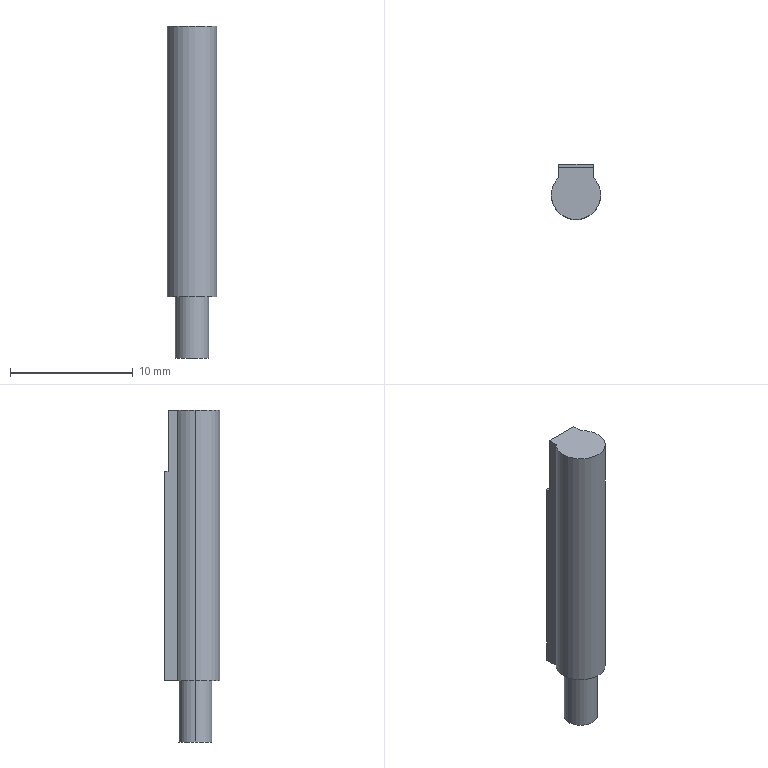Part | SolidWorks | features ICE 3, RefAxis 3, 3DProfileFeature 1, Extrusion 1, Revolution 1 | 1 solid | 23 faces | box 4 x 4.5 x 27 mm | volume 342.413 mm3 | plane 13 | cylinder 10 | commonest cylinder face diameters 2.1 x3 4 x3 2.5 x2 2.7 x2
STEP:
#1=CARTESIAN_POINT('',(1.35,0.,-27.));
#2=VERTEX_POINT('',#1);
#3=CARTESIAN_POINT('',(-1.35,0.,-27.));
#4=VERTEX_POINT('',#3);
#5=CARTESIAN_POINT('',(0.,0.,-27.));
#6=DIRECTION('',(0.,0.,1.));
#7=DIRECTION('',(1.,0.,0.));
#8=AXIS2_PLACEMENT_3D('',#5,#6,#7);
#9=CIRCLE('',#8,1.35);
#10=EDGE_CURVE('',#2,#4,#9,.T.);
#11=ORIENTED_EDGE('',*,*,#10,.T.);
#12=CARTESIAN_POINT('',(-1.35,0.,-22.));
#13=VERTEX_POINT('',#12);
#14=CARTESIAN_POINT('',(-1.35,0.,-27.));
#15=DIRECTION('',(0.,0.,1.));
#16=VECTOR('',#15,1000.);
#17=LINE('',#14,#16);
#18=EDGE_CURVE('',#4,#13,#17,.T.);
#19=ORIENTED_EDGE('',*,*,#18,.T.);
#20=CARTESIAN_POINT('',(1.35,0.,-22.));
#21=VERTEX_POINT('',#20);
#22=CARTESIAN_POINT('',(0.,0.,-22.));
#23=DIRECTION('',(0.,0.,-1.));
#24=DIRECTION('',(1.,0.,0.));
#25=AXIS2_PLACEMENT_3D('',#22,#23,#24);
#26=CIRCLE('',#25,1.35);
#27=EDGE_CURVE('',#13,#21,#26,.T.);
#28=ORIENTED_EDGE('',*,*,#27,.T.);
#29=CARTESIAN_POINT('',(1.35,0.,-27.));
#30=DIRECTION('',(0.,0.,1.));
#31=VECTOR('',#30,1000.);
#32=LINE('',#29,#31);
#33=EDGE_CURVE('',#2,#21,#32,.T.);
#34=ORIENTED_EDGE('',*,*,#33,.F.);
#35=EDGE_LOOP('',(#11,#19,#28,#34));
#36=FACE_OUTER_BOUND('',#35,.T.);
#37=CARTESIAN_POINT('',(0.,0.,-27.));
#38=DIRECTION('',(0.,0.,1.));
#39=DIRECTION('',(1.,0.,0.));
#40=AXIS2_PLACEMENT_3D('',#37,#38,#39);
#41=CYLINDRICAL_SURFACE('',#40,1.35);
#42=ADVANCED_FACE('',(#36),#41,.T.);
#43=CARTESIAN_POINT('',(-0.5443,2.1,-1.102));
#44=VERTEX_POINT('',#43);
#45=CARTESIAN_POINT('',(0.,2.1,-0.95));
#46=VERTEX_POINT('',#45);
#47=CARTESIAN_POINT('',(0.,2.1,-2.));
#48=DIRECTION('',(0.,1.,0.));
#49=DIRECTION('',(0.,0.,1.));
#50=AXIS2_PLACEMENT_3D('',#47,#48,#49);
#51=CIRCLE('',#50,1.05);
#52=EDGE_CURVE('',#44,#46,#51,.T.);
#53=ORIENTED_EDGE('',*,*,#52,.T.);
#54=CARTESIAN_POINT('',(0.,2.2,-0.95));
#55=VERTEX_POINT('',#54);
#56=CARTESIAN_POINT('',(0.,2.1,-0.95));
#57=DIRECTION('',(0.,1.,0.));
#58=VECTOR('',#57,1000.);
#59=LINE('',#56,#58);
#60=EDGE_CURVE('',#46,#55,#59,.T.);
#61=ORIENTED_EDGE('',*,*,#60,.T.);
#62=CARTESIAN_POINT('',(-0.5443,2.2,-1.102));
#63=VERTEX_POINT('',#62);
#64=CARTESIAN_POINT('',(0.,2.2,-2.));
#65=DIRECTION('',(0.,1.,0.));
#66=DIRECTION('',(0.,0.,1.));
#67=AXIS2_PLACEMENT_3D('',#64,#65,#66);
#68=CIRCLE('',#67,1.05);
#69=EDGE_CURVE('',#63,#55,#68,.T.);
#70=ORIENTED_EDGE('',*,*,#69,.F.);
#71=CARTESIAN_POINT('',(-0.5443,2.1,-1.102));
#72=DIRECTION('',(0.,1.,0.));
#73=VECTOR('',#72,1000.);
#74=LINE('',#71,#73);
#75=EDGE_CURVE('',#44,#63,#74,.T.);
#76=ORIENTED_EDGE('',*,*,#75,.F.);
#77=EDGE_LOOP('',(#53,#61,#70,#76));
#78=FACE_OUTER_BOUND('',#77,.T.);
#79=CARTESIAN_POINT('',(0.,2.1,-2.));
#80=DIRECTION('',(0.,1.,0.));
#81=DIRECTION('',(0.,0.,1.));
#82=AXIS2_PLACEMENT_3D('',#79,#80,#81);
#83=CYLINDRICAL_SURFACE('',#82,1.05);
#84=ADVANCED_FACE('',(#78),#83,.T.);
#85=CARTESIAN_POINT('',(0.,2.1,-3.25));
#86=VERTEX_POINT('',#85);
#87=CARTESIAN_POINT('',(0.,2.1,-0.75));
#88=VERTEX_POINT('',#87);
#89=CARTESIAN_POINT('',(0.,2.1,-2.));
#90=DIRECTION('',(0.,1.,0.));
#91=DIRECTION('',(0.,0.,1.));
#92=AXIS2_PLACEMENT_3D('',#89,#90,#91);
#93=CIRCLE('',#92,1.25);
#94=EDGE_CURVE('',#86,#88,#93,.T.);
#95=ORIENTED_EDGE('',*,*,#94,.F.);
#96=CARTESIAN_POINT('',(0.,2.2,-3.25));
#97=VERTEX_POINT('',#96);
#98=CARTESIAN_POINT('',(0.,2.1,-3.25));
#99=DIRECTION('',(0.,1.,0.));
#100=VECTOR('',#99,1000.);
#101=LINE('',#98,#100);
#102=EDGE_CURVE('',#86,#97,#101,.T.);
#103=ORIENTED_EDGE('',*,*,#102,.T.);
#104=CARTESIAN_POINT('',(0.,2.2,-0.75));
#105=VERTEX_POINT('',#104);
#106=CARTESIAN_POINT('',(0.,2.2,-2.));
#107=DIRECTION('',(0.,1.,0.));
#108=DIRECTION('',(0.,0.,1.));
#109=AXIS2_PLACEMENT_3D('',#106,#107,#108);
#110=CIRCLE('',#109,1.25);
#111=EDGE_CURVE('',#97,#105,#110,.T.);
#112=ORIENTED_EDGE('',*,*,#111,.T.);
#113=CARTESIAN_POINT('',(0.,2.1,-0.75));
#114=DIRECTION('',(0.,1.,0.));
#115=VECTOR('',#114,1000.);
#116=LINE('',#113,#115);
#117=EDGE_CURVE('',#88,#105,#116,.T.);
#118=ORIENTED_EDGE('',*,*,#117,.F.);
#119=EDGE_LOOP('',(#95,#103,#112,#118));
#120=FACE_OUTER_BOUND('',#119,.T.);
#121=CARTESIAN_POINT('',(0.,2.1,-2.));
#122=DIRECTION('',(0.,1.,0.));
#123=DIRECTION('',(0.,0.,1.));
#124=AXIS2_PLACEMENT_3D('',#121,#122,#123);
#125=CYLINDRICAL_SURFACE('',#124,1.25);
#126=ADVANCED_FACE('',(#120),#125,.F.);
#127=CARTESIAN_POINT('',(-1.4,1.428,-22.));
#128=VERTEX_POINT('',#127);
#129=CARTESIAN_POINT('',(-2.,0.,-22.));
#130=VERTEX_POINT('',#129);
#131=CARTESIAN_POINT('',(0.,0.,-22.));
#132=DIRECTION('',(0.,0.,1.));
#133=DIRECTION('',(1.,0.,0.));
#134=AXIS2_PLACEMENT_3D('',#131,#132,#133);
#135=CIRCLE('',#134,2.);
#136=EDGE_CURVE('',#128,#130,#135,.T.);
#137=ORIENTED_EDGE('',*,*,#136,.T.);
#138=CARTESIAN_POINT('',(-2.,0.,0.));
#139=VERTEX_POINT('',#138);
#140=CARTESIAN_POINT('',(-2.,0.,-22.));
#141=DIRECTION('',(0.,0.,1.));
#142=VECTOR('',#141,1000.);
#143=LINE('',#140,#142);
#144=EDGE_CURVE('',#130,#139,#143,.T.);
#145=ORIENTED_EDGE('',*,*,#144,.T.);
#146=CARTESIAN_POINT('',(-1.4,1.428,0.));
#147=VERTEX_POINT('',#146);
#148=CARTESIAN_POINT('',(0.,0.,0.));
#149=DIRECTION('',(0.,0.,1.));
#150=DIRECTION('',(1.,0.,0.));
#151=AXIS2_PLACEMENT_3D('',#148,#149,#150);
#152=CIRCLE('',#151,2.);
#153=EDGE_CURVE('',#147,#139,#152,.T.);
#154=ORIENTED_EDGE('',*,*,#153,.F.);
#155=CARTESIAN_POINT('',(-1.4,1.428,-22.));
#156=DIRECTION('',(0.,0.,1.));
#157=VECTOR('',#156,1000.);
#158=LINE('',#155,#157);
#159=EDGE_CURVE('',#128,#147,#158,.T.);
#160=ORIENTED_EDGE('',*,*,#159,.F.);
#161=EDGE_LOOP('',(#137,#145,#154,#160));
#162=FACE_OUTER_BOUND('',#161,.T.);
#163=CARTESIAN_POINT('',(0.,0.,-22.));
#164=DIRECTION('',(0.,0.,1.));
#165=DIRECTION('',(1.,0.,0.));
#166=AXIS2_PLACEMENT_3D('',#163,#164,#165);
#167=CYLINDRICAL_SURFACE('',#166,2.);
#168=ADVANCED_FACE('',(#162),#167,.T.);
#169=ORIENTED_EDGE('',*,*,#144,.F.);
#170=CARTESIAN_POINT('',(2.,0.,-22.));
#171=VERTEX_POINT('',#170);
#172=CARTESIAN_POINT('',(0.,0.,-22.));
#173=DIRECTION('',(0.,0.,1.));
#174=DIRECTION('',(1.,0.,0.));
#175=AXIS2_PLACEMENT_3D('',#172,#173,#174);
#176=CIRCLE('',#175,2.);
#177=EDGE_CURVE('',#130,#171,#176,.T.);
#178=ORIENTED_EDGE('',*,*,#177,.T.);
#179=CARTESIAN_POINT('',(2.,0.,0.));
#180=VERTEX_POINT('',#179);
#181=CARTESIAN_POINT('',(2.,0.,-22.));
#182=DIRECTION('',(0.,0.,1.));
#183=VECTOR('',#182,1000.);
#184=LINE('',#181,#183);
#185=EDGE_CURVE('',#171,#180,#184,.T.);
#186=ORIENTED_EDGE('',*,*,#185,.T.);
#187=CARTESIAN_POINT('',(0.,0.,0.));
#188=DIRECTION('',(0.,0.,1.));
#189=DIRECTION('',(1.,0.,0.));
#190=AXIS2_PLACEMENT_3D('',#187,#188,#189);
#191=CIRCLE('',#190,2.);
#192=EDGE_CURVE('',#139,#180,#191,.T.);
#193=ORIENTED_EDGE('',*,*,#192,.F.);
#194=EDGE_LOOP('',(#169,#178,#186,#193));
#195=FACE_OUTER_BOUND('',#194,.T.);
#196=CARTESIAN_POINT('',(0.,0.,-22.));
#197=DIRECTION('',(0.,0.,1.));
#198=DIRECTION('',(1.,0.,0.));
#199=AXIS2_PLACEMENT_3D('',#196,#197,#198);
#200=CYLINDRICAL_SURFACE('',#199,2.);
#201=ADVANCED_FACE('',(#195),#200,.T.);
#202=ORIENTED_EDGE('',*,*,#136,.F.);
#203=CARTESIAN_POINT('',(-1.4,2.5,-22.));
#204=VERTEX_POINT('',#203);
#205=CARTESIAN_POINT('',(-1.4,2.5,-22.));
#206=DIRECTION('',(0.,-1.,0.));
#207=VECTOR('',#206,1000.);
#208=LINE('',#205,#207);
#209=EDGE_CURVE('',#204,#128,#208,.T.);
#210=ORIENTED_EDGE('',*,*,#209,.F.);
#211=CARTESIAN_POINT('',(1.4,2.5,-22.));
#212=VERTEX_POINT('',#211);
#213=CARTESIAN_POINT('',(1.4,2.5,-22.));
#214=DIRECTION('',(-1.,0.,0.));
#215=VECTOR('',#214,1000.);
#216=LINE('',#213,#215);
#217=EDGE_CURVE('',#212,#204,#216,.T.);
#218=ORIENTED_EDGE('',*,*,#217,.F.);
#219=CARTESIAN_POINT('',(1.4,1.428,-22.));
#220=VERTEX_POINT('',#219);
#221=CARTESIAN_POINT('',(1.4,1.428,-22.));
#222=DIRECTION('',(0.,1.,0.));
#223=VECTOR('',#222,1000.);
#224=LINE('',#221,#223);
#225=EDGE_CURVE('',#220,#212,#224,.T.);
#226=ORIENTED_EDGE('',*,*,#225,.F.);
#227=CARTESIAN_POINT('',(0.,0.,-22.));
#228=DIRECTION('',(0.,0.,1.));
#229=DIRECTION('',(1.,0.,0.));
#230=AXIS2_PLACEMENT_3D('',#227,#228,#229);
#231=CIRCLE('',#230,2.);
#232=EDGE_CURVE('',#171,#220,#231,.T.);
#233=ORIENTED_EDGE('',*,*,#232,.F.);
#234=ORIENTED_EDGE('',*,*,#177,.F.);
#235=EDGE_LOOP('',(#202,#210,#218,#226,#233,#234));
#236=FACE_OUTER_BOUND('',#235,.T.);
#237=CARTESIAN_POINT('',(0.,0.,-22.));
#238=DIRECTION('',(0.,0.,-1.));
#239=DIRECTION('',(1.,0.,0.));
#240=AXIS2_PLACEMENT_3D('',#237,#238,#239);
#241=CIRCLE('',#240,1.35);
#242=EDGE_CURVE('',#21,#13,#241,.T.);
#243=ORIENTED_EDGE('',*,*,#242,.F.);
#244=ORIENTED_EDGE('',*,*,#27,.F.);
#245=EDGE_LOOP('',(#243,#244));
#246=FACE_BOUND('',#245,.T.);
#247=CARTESIAN_POINT('',(0.,0.,-22.));
#248=DIRECTION('',(0.,0.,1.));
#249=DIRECTION('',(1.,0.,0.));
#250=AXIS2_PLACEMENT_3D('',#247,#248,#249);
#251=PLANE('',#250);
#252=ADVANCED_FACE('',(#236,#246),#251,.F.);
#253=CARTESIAN_POINT('',(-0.8979,2.1,-1.456));
#254=VERTEX_POINT('',#253);
#255=CARTESIAN_POINT('',(-0.8979,2.2,-1.456));
#256=VERTEX_POINT('',#255);
#257=CARTESIAN_POINT('',(-0.8979,2.1,-1.456));
#258=DIRECTION('',(0.,1.,0.));
#259=VECTOR('',#258,1000.);
#260=LINE('',#257,#259);
#261=EDGE_CURVE('',#254,#256,#260,.T.);
#262=ORIENTED_EDGE('',*,*,#261,.T.);
#263=CARTESIAN_POINT('',(0.5443,2.2,-2.898));
#264=VERTEX_POINT('',#263);
#265=CARTESIAN_POINT('',(0.,2.2,-2.));
#266=DIRECTION('',(0.,1.,0.));
#267=DIRECTION('',(0.,0.,1.));
#268=AXIS2_PLACEMENT_3D('',#265,#266,#267);
#269=CIRCLE('',#268,1.05);
#270=EDGE_CURVE('',#264,#256,#269,.T.);
#271=ORIENTED_EDGE('',*,*,#270,.F.);
#272=CARTESIAN_POINT('',(0.5443,2.1,-2.898));
#273=VERTEX_POINT('',#272);
#274=CARTESIAN_POINT('',(0.5443,2.1,-2.898));
#275=DIRECTION('',(0.,1.,0.));
#276=VECTOR('',#275,1000.);
#277=LINE('',#274,#276);
#278=EDGE_CURVE('',#273,#264,#277,.T.);
#279=ORIENTED_EDGE('',*,*,#278,.F.);
#280=CARTESIAN_POINT('',(0.,2.1,-2.));
#281=DIRECTION('',(0.,1.,0.));
#282=DIRECTION('',(0.,0.,1.));
#283=AXIS2_PLACEMENT_3D('',#280,#281,#282);
#284=CIRCLE('',#283,1.05);
#285=EDGE_CURVE('',#273,#254,#284,.T.);
#286=ORIENTED_EDGE('',*,*,#285,.T.);
#287=EDGE_LOOP('',(#262,#271,#279,#286));
#288=FACE_OUTER_BOUND('',#287,.T.);
#289=CARTESIAN_POINT('',(0.,2.1,-2.));
#290=DIRECTION('',(0.,1.,0.));
#291=DIRECTION('',(0.,0.,1.));
#292=AXIS2_PLACEMENT_3D('',#289,#290,#291);
#293=CYLINDRICAL_SURFACE('',#292,1.05);
#294=ADVANCED_FACE('',(#288),#293,.T.);
#295=ORIENTED_EDGE('',*,*,#270,.T.);
#296=CARTESIAN_POINT('',(0.5443,2.2,-2.898));
#297=DIRECTION('',(-0.7071,0.,0.7071));
#298=VECTOR('',#297,1000.);
#299=LINE('',#296,#298);
#300=EDGE_CURVE('',#264,#256,#299,.T.);
#301=ORIENTED_EDGE('',*,*,#300,.F.);
#302=EDGE_LOOP('',(#295,#301));
#303=FACE_OUTER_BOUND('',#302,.T.);
#304=CARTESIAN_POINT('',(-1.4,2.2,-5.));
#305=DIRECTION('',(0.,-1.,0.));
#306=DIRECTION('',(0.,0.,-1.));
#307=AXIS2_PLACEMENT_3D('',#304,#305,#306);
#308=PLANE('',#307);
#309=ADVANCED_FACE('',(#303),#308,.F.);
#310=CARTESIAN_POINT('',(-1.4,2.5,-5.));
#311=VERTEX_POINT('',#310);
#312=CARTESIAN_POINT('',(-1.4,2.5,-22.));
#313=DIRECTION('',(0.,0.,1.));
#314=VECTOR('',#313,1000.);
#315=LINE('',#312,#314);
#316=EDGE_CURVE('',#204,#311,#315,.T.);
#317=ORIENTED_EDGE('',*,*,#316,.T.);
#318=CARTESIAN_POINT('',(1.4,2.5,-5.));
#319=VERTEX_POINT('',#318);
#320=CARTESIAN_POINT('',(1.4,2.5,-5.));
#321=DIRECTION('',(-1.,0.,0.));
#322=VECTOR('',#321,1000.);
#323=LINE('',#320,#322);
#324=EDGE_CURVE('',#319,#311,#323,.T.);
#325=ORIENTED_EDGE('',*,*,#324,.F.);
#326=CARTESIAN_POINT('',(1.4,2.5,-22.));
#327=DIRECTION('',(0.,0.,1.));
#328=VECTOR('',#327,1000.);
#329=LINE('',#326,#328);
#330=EDGE_CURVE('',#212,#319,#329,.T.);
#331=ORIENTED_EDGE('',*,*,#330,.F.);
#332=ORIENTED_EDGE('',*,*,#217,.T.);
#333=EDGE_LOOP('',(#317,#325,#331,#332));
#334=FACE_OUTER_BOUND('',#333,.T.);
#335=CARTESIAN_POINT('',(1.4,2.5,-22.));
#336=DIRECTION('',(0.,1.,0.));
#337=DIRECTION('',(0.,0.,1.));
#338=AXIS2_PLACEMENT_3D('',#335,#336,#337);
#339=PLANE('',#338);
#340=ADVANCED_FACE('',(#334),#339,.T.);
#341=ORIENTED_EDGE('',*,*,#185,.F.);
#342=ORIENTED_EDGE('',*,*,#232,.T.);
#343=CARTESIAN_POINT('',(1.4,1.428,0.));
#344=VERTEX_POINT('',#343);
#345=CARTESIAN_POINT('',(1.4,1.428,-22.));
#346=DIRECTION('',(0.,0.,1.));
#347=VECTOR('',#346,1000.);
#348=LINE('',#345,#347);
#349=EDGE_CURVE('',#220,#344,#348,.T.);
#350=ORIENTED_EDGE('',*,*,#349,.T.);
#351=CARTESIAN_POINT('',(0.,0.,0.));
#352=DIRECTION('',(0.,0.,1.));
#353=DIRECTION('',(1.,0.,0.));
#354=AXIS2_PLACEMENT_3D('',#351,#352,#353);
#355=CIRCLE('',#354,2.);
#356=EDGE_CURVE('',#180,#344,#355,.T.);
#357=ORIENTED_EDGE('',*,*,#356,.F.);
#358=EDGE_LOOP('',(#341,#342,#350,#357));
#359=FACE_OUTER_BOUND('',#358,.T.);
#360=CARTESIAN_POINT('',(0.,0.,-22.));
#361=DIRECTION('',(0.,0.,1.));
#362=DIRECTION('',(1.,0.,0.));
#363=AXIS2_PLACEMENT_3D('',#360,#361,#362);
#364=CYLINDRICAL_SURFACE('',#363,2.);
#365=ADVANCED_FACE('',(#359),#364,.T.);
#366=CARTESIAN_POINT('',(-1.4,2.2,-5.));
#367=VERTEX_POINT('',#366);
#368=CARTESIAN_POINT('',(-1.4,2.2,0.));
#369=VERTEX_POINT('',#368);
#370=CARTESIAN_POINT('',(-1.4,2.2,-5.));
#371=DIRECTION('',(0.,0.,1.));
#372=VECTOR('',#371,1000.);
#373=LINE('',#370,#372);
#374=EDGE_CURVE('',#367,#369,#373,.T.);
#375=ORIENTED_EDGE('',*,*,#374,.F.);
#376=CARTESIAN_POINT('',(-1.4,2.5,-5.));
#377=DIRECTION('',(0.,-1.,0.));
#378=VECTOR('',#377,1000.);
#379=LINE('',#376,#378);
#380=EDGE_CURVE('',#311,#367,#379,.T.);
#381=ORIENTED_EDGE('',*,*,#380,.F.);
#382=ORIENTED_EDGE('',*,*,#316,.F.);
#383=ORIENTED_EDGE('',*,*,#209,.T.);
#384=ORIENTED_EDGE('',*,*,#159,.T.);
#385=CARTESIAN_POINT('',(-1.4,2.5,0.));
#386=DIRECTION('',(0.,-1.,0.));
#387=VECTOR('',#386,1000.);
#388=LINE('',#385,#387);
#389=EDGE_CURVE('',#369,#147,#388,.T.);
#390=ORIENTED_EDGE('',*,*,#389,.F.);
#391=EDGE_LOOP('',(#375,#381,#382,#383,#384,#390));
#392=FACE_OUTER_BOUND('',#391,.T.);
#393=CARTESIAN_POINT('',(-1.4,2.5,-22.));
#394=DIRECTION('',(-1.,0.,0.));
#395=DIRECTION('',(0.,0.,1.));
#396=AXIS2_PLACEMENT_3D('',#393,#394,#395);
#397=PLANE('',#396);
#398=ADVANCED_FACE('',(#392),#397,.T.);
#399=CARTESIAN_POINT('',(1.4,2.2,-5.));
#400=VERTEX_POINT('',#399);
#401=CARTESIAN_POINT('',(1.4,2.2,0.));
#402=VERTEX_POINT('',#401);
#403=CARTESIAN_POINT('',(1.4,2.2,-5.));
#404=DIRECTION('',(0.,0.,1.));
#405=VECTOR('',#404,1000.);
#406=LINE('',#403,#405);
#407=EDGE_CURVE('',#400,#402,#406,.T.);
#408=ORIENTED_EDGE('',*,*,#407,.T.);
#409=CARTESIAN_POINT('',(1.4,1.428,0.));
#410=DIRECTION('',(0.,1.,0.));
#411=VECTOR('',#410,1000.);
#412=LINE('',#409,#411);
#413=EDGE_CURVE('',#344,#402,#412,.T.);
#414=ORIENTED_EDGE('',*,*,#413,.F.);
#415=ORIENTED_EDGE('',*,*,#349,.F.);
#416=ORIENTED_EDGE('',*,*,#225,.T.);
#417=ORIENTED_EDGE('',*,*,#330,.T.);
#418=CARTESIAN_POINT('',(1.4,2.2,-5.));
#419=DIRECTION('',(0.,1.,0.));
#420=VECTOR('',#419,1000.);
#421=LINE('',#418,#420);
#422=EDGE_CURVE('',#400,#319,#421,.T.);
#423=ORIENTED_EDGE('',*,*,#422,.F.);
#424=EDGE_LOOP('',(#408,#414,#415,#416,#417,#423));
#425=FACE_OUTER_BOUND('',#424,.T.);
#426=CARTESIAN_POINT('',(1.4,1.428,-22.));
#427=DIRECTION('',(1.,0.,0.));
#428=DIRECTION('',(0.,0.,-1.));
#429=AXIS2_PLACEMENT_3D('',#426,#427,#428);
#430=PLANE('',#429);
#431=ADVANCED_FACE('',(#425),#430,.T.);
#432=CARTESIAN_POINT('',(-1.4,2.2,0.));
#433=DIRECTION('',(1.,0.,0.));
#434=VECTOR('',#433,1000.);
#435=LINE('',#432,#434);
#436=EDGE_CURVE('',#369,#402,#435,.T.);
#437=ORIENTED_EDGE('',*,*,#436,.F.);
#438=ORIENTED_EDGE('',*,*,#389,.T.);
#439=ORIENTED_EDGE('',*,*,#153,.T.);
#440=ORIENTED_EDGE('',*,*,#192,.T.);
#441=ORIENTED_EDGE('',*,*,#356,.T.);
#442=ORIENTED_EDGE('',*,*,#413,.T.);
#443=EDGE_LOOP('',(#437,#438,#439,#440,#441,#442));
#444=FACE_OUTER_BOUND('',#443,.T.);
#445=CARTESIAN_POINT('',(0.,0.,0.));
#446=DIRECTION('',(0.,0.,1.));
#447=DIRECTION('',(1.,0.,0.));
#448=AXIS2_PLACEMENT_3D('',#445,#446,#447);
#449=PLANE('',#448);
#450=ADVANCED_FACE('',(#444),#449,.T.);
#451=CARTESIAN_POINT('',(0.,2.2,-2.));
#452=DIRECTION('',(0.,1.,0.));
#453=DIRECTION('',(0.,0.,1.));
#454=AXIS2_PLACEMENT_3D('',#451,#452,#453);
#455=CIRCLE('',#454,1.25);
#456=EDGE_CURVE('',#105,#97,#455,.T.);
#457=ORIENTED_EDGE('',*,*,#456,.F.);
#458=ORIENTED_EDGE('',*,*,#111,.F.);
#459=EDGE_LOOP('',(#457,#458));
#460=FACE_BOUND('',#459,.T.);
#461=ORIENTED_EDGE('',*,*,#436,.T.);
#462=ORIENTED_EDGE('',*,*,#407,.F.);
#463=CARTESIAN_POINT('',(-1.4,2.2,-5.));
#464=DIRECTION('',(1.,0.,0.));
#465=VECTOR('',#464,1000.);
#466=LINE('',#463,#465);
#467=EDGE_CURVE('',#367,#400,#466,.T.);
#468=ORIENTED_EDGE('',*,*,#467,.F.);
#469=ORIENTED_EDGE('',*,*,#374,.T.);
#470=EDGE_LOOP('',(#461,#462,#468,#469));
#471=FACE_OUTER_BOUND('',#470,.T.);
#472=CARTESIAN_POINT('',(-1.4,2.2,-5.));
#473=DIRECTION('',(0.,-1.,0.));
#474=DIRECTION('',(0.,0.,-1.));
#475=AXIS2_PLACEMENT_3D('',#472,#473,#474);
#476=PLANE('',#475);
#477=ADVANCED_FACE('',(#460,#471),#476,.F.);
#478=ORIENTED_EDGE('',*,*,#324,.T.);
#479=ORIENTED_EDGE('',*,*,#380,.T.);
#480=ORIENTED_EDGE('',*,*,#467,.T.);
#481=ORIENTED_EDGE('',*,*,#422,.T.);
#482=EDGE_LOOP('',(#478,#479,#480,#481));
#483=FACE_OUTER_BOUND('',#482,.T.);
#484=CARTESIAN_POINT('',(0.,0.,-5.));
#485=DIRECTION('',(0.,0.,1.));
#486=DIRECTION('',(1.,0.,0.));
#487=AXIS2_PLACEMENT_3D('',#484,#485,#486);
#488=PLANE('',#487);
#489=ADVANCED_FACE('',(#483),#488,.T.);
#490=ORIENTED_EDGE('',*,*,#102,.F.);
#491=CARTESIAN_POINT('',(0.,2.1,-2.));
#492=DIRECTION('',(0.,1.,0.));
#493=DIRECTION('',(0.,0.,1.));
#494=AXIS2_PLACEMENT_3D('',#491,#492,#493);
#495=CIRCLE('',#494,1.25);
#496=EDGE_CURVE('',#88,#86,#495,.T.);
#497=ORIENTED_EDGE('',*,*,#496,.F.);
#498=ORIENTED_EDGE('',*,*,#117,.T.);
#499=ORIENTED_EDGE('',*,*,#456,.T.);
#500=EDGE_LOOP('',(#490,#497,#498,#499));
#501=FACE_OUTER_BOUND('',#500,.T.);
#502=CARTESIAN_POINT('',(0.,2.1,-2.));
#503=DIRECTION('',(0.,1.,0.));
#504=DIRECTION('',(0.,0.,1.));
#505=AXIS2_PLACEMENT_3D('',#502,#503,#504);
#506=CYLINDRICAL_SURFACE('',#505,1.25);
#507=ADVANCED_FACE('',(#501),#506,.F.);
#508=ORIENTED_EDGE('',*,*,#52,.F.);
#509=CARTESIAN_POINT('',(0.8979,2.1,-2.544));
#510=VERTEX_POINT('',#509);
#511=CARTESIAN_POINT('',(-0.5443,2.1,-1.102));
#512=DIRECTION('',(0.7071,0.,-0.7071));
#513=VECTOR('',#512,1000.);
#514=LINE('',#511,#513);
#515=EDGE_CURVE('',#44,#510,#514,.T.);
#516=ORIENTED_EDGE('',*,*,#515,.T.);
#517=CARTESIAN_POINT('',(0.,2.1,-2.));
#518=DIRECTION('',(0.,1.,0.));
#519=DIRECTION('',(0.,0.,1.));
#520=AXIS2_PLACEMENT_3D('',#517,#518,#519);
#521=CIRCLE('',#520,1.05);
#522=EDGE_CURVE('',#46,#510,#521,.T.);
#523=ORIENTED_EDGE('',*,*,#522,.F.);
#524=EDGE_LOOP('',(#508,#516,#523));
#525=FACE_BOUND('',#524,.T.);
#526=ORIENTED_EDGE('',*,*,#285,.F.);
#527=CARTESIAN_POINT('',(0.5443,2.1,-2.898));
#528=DIRECTION('',(-0.7071,0.,0.7071));
#529=VECTOR('',#528,1000.);
#530=LINE('',#527,#529);
#531=EDGE_CURVE('',#273,#254,#530,.T.);
#532=ORIENTED_EDGE('',*,*,#531,.T.);
#533=EDGE_LOOP('',(#526,#532));
#534=FACE_BOUND('',#533,.T.);
#535=ORIENTED_EDGE('',*,*,#496,.T.);
#536=ORIENTED_EDGE('',*,*,#94,.T.);
#537=EDGE_LOOP('',(#535,#536));
#538=FACE_OUTER_BOUND('',#537,.T.);
#539=CARTESIAN_POINT('',(0.,2.1,-2.));
#540=DIRECTION('',(0.,1.,0.));
#541=DIRECTION('',(0.,0.,1.));
#542=AXIS2_PLACEMENT_3D('',#539,#540,#541);
#543=PLANE('',#542);
#544=ADVANCED_FACE('',(#525,#534,#538),#543,.T.);
#545=ORIENTED_EDGE('',*,*,#60,.F.);
#546=ORIENTED_EDGE('',*,*,#522,.T.);
#547=CARTESIAN_POINT('',(0.8979,2.2,-2.544));
#548=VERTEX_POINT('',#547);
#549=CARTESIAN_POINT('',(0.8979,2.1,-2.544));
#550=DIRECTION('',(0.,1.,0.));
#551=VECTOR('',#550,1000.);
#552=LINE('',#549,#551);
#553=EDGE_CURVE('',#510,#548,#552,.T.);
#554=ORIENTED_EDGE('',*,*,#553,.T.);
#555=CARTESIAN_POINT('',(0.,2.2,-2.));
#556=DIRECTION('',(0.,1.,0.));
#557=DIRECTION('',(0.,0.,1.));
#558=AXIS2_PLACEMENT_3D('',#555,#556,#557);
#559=CIRCLE('',#558,1.05);
#560=EDGE_CURVE('',#55,#548,#559,.T.);
#561=ORIENTED_EDGE('',*,*,#560,.F.);
#562=EDGE_LOOP('',(#545,#546,#554,#561));
#563=FACE_OUTER_BOUND('',#562,.T.);
#564=CARTESIAN_POINT('',(0.,2.1,-2.));
#565=DIRECTION('',(0.,1.,0.));
#566=DIRECTION('',(0.,0.,1.));
#567=AXIS2_PLACEMENT_3D('',#564,#565,#566);
#568=CYLINDRICAL_SURFACE('',#567,1.05);
#569=ADVANCED_FACE('',(#563),#568,.T.);
#570=ORIENTED_EDGE('',*,*,#69,.T.);
#571=ORIENTED_EDGE('',*,*,#560,.T.);
#572=CARTESIAN_POINT('',(-0.5443,2.2,-1.102));
#573=DIRECTION('',(0.7071,0.,-0.7071));
#574=VECTOR('',#573,1000.);
#575=LINE('',#572,#574);
#576=EDGE_CURVE('',#63,#548,#575,.T.);
#577=ORIENTED_EDGE('',*,*,#576,.F.);
#578=EDGE_LOOP('',(#570,#571,#577));
#579=FACE_OUTER_BOUND('',#578,.T.);
#580=CARTESIAN_POINT('',(-1.4,2.2,-5.));
#581=DIRECTION('',(0.,-1.,0.));
#582=DIRECTION('',(0.,0.,-1.));
#583=AXIS2_PLACEMENT_3D('',#580,#581,#582);
#584=PLANE('',#583);
#585=ADVANCED_FACE('',(#579),#584,.F.);
#586=ORIENTED_EDGE('',*,*,#300,.T.);
#587=ORIENTED_EDGE('',*,*,#261,.F.);
#588=ORIENTED_EDGE('',*,*,#531,.F.);
#589=ORIENTED_EDGE('',*,*,#278,.T.);
#590=EDGE_LOOP('',(#586,#587,#588,#589));
#591=FACE_OUTER_BOUND('',#590,.T.);
#592=CARTESIAN_POINT('',(0.5443,2.1,-2.898));
#593=DIRECTION('',(-0.7071,0.,-0.7071));
#594=DIRECTION('',(-0.7071,0.,0.7071));
#595=AXIS2_PLACEMENT_3D('',#592,#593,#594);
#596=PLANE('',#595);
#597=ADVANCED_FACE('',(#591),#596,.F.);
#598=ORIENTED_EDGE('',*,*,#576,.T.);
#599=ORIENTED_EDGE('',*,*,#553,.F.);
#600=ORIENTED_EDGE('',*,*,#515,.F.);
#601=ORIENTED_EDGE('',*,*,#75,.T.);
#602=EDGE_LOOP('',(#598,#599,#600,#601));
#603=FACE_OUTER_BOUND('',#602,.T.);
#604=CARTESIAN_POINT('',(-0.5443,2.1,-1.102));
#605=DIRECTION('',(0.7071,0.,0.7071));
#606=DIRECTION('',(0.7071,0.,-0.7071));
#607=AXIS2_PLACEMENT_3D('',#604,#605,#606);
#608=PLANE('',#607);
#609=ADVANCED_FACE('',(#603),#608,.F.);
#610=ORIENTED_EDGE('',*,*,#18,.F.);
#611=CARTESIAN_POINT('',(0.,0.,-27.));
#612=DIRECTION('',(0.,0.,1.));
#613=DIRECTION('',(1.,0.,0.));
#614=AXIS2_PLACEMENT_3D('',#611,#612,#613);
#615=CIRCLE('',#614,1.35);
#616=EDGE_CURVE('',#4,#2,#615,.T.);
#617=ORIENTED_EDGE('',*,*,#616,.T.);
#618=ORIENTED_EDGE('',*,*,#33,.T.);
#619=ORIENTED_EDGE('',*,*,#242,.T.);
#620=EDGE_LOOP('',(#610,#617,#618,#619));
#621=FACE_OUTER_BOUND('',#620,.T.);
#622=CARTESIAN_POINT('',(0.,0.,-27.));
#623=DIRECTION('',(0.,0.,1.));
#624=DIRECTION('',(1.,0.,0.));
#625=AXIS2_PLACEMENT_3D('',#622,#623,#624);
#626=CYLINDRICAL_SURFACE('',#625,1.35);
#627=ADVANCED_FACE('',(#621),#626,.T.);
#628=ORIENTED_EDGE('',*,*,#10,.F.);
#629=ORIENTED_EDGE('',*,*,#616,.F.);
#630=EDGE_LOOP('',(#628,#629));
#631=FACE_OUTER_BOUND('',#630,.T.);
#632=CARTESIAN_POINT('',(-1.35,0.,-27.));
#633=DIRECTION('',(0.,0.,1.));
#634=DIRECTION('',(1.,0.,0.));
#635=AXIS2_PLACEMENT_3D('',#632,#633,#634);
#636=PLANE('',#635);
#637=ADVANCED_FACE('',(#631),#636,.F.);
#638=CLOSED_SHELL('',(#42,#84,#126,#168,#201,#252,#294,#309,#340,#365,#398,#431,#450,#477,#489,#507,#544,#569,#585,#597,#609,#627,#637));
#639=MANIFOLD_SOLID_BREP('',#638);
#640=CARTESIAN_POINT('',(0.,0.,0.));
#641=DIRECTION('',(0.,0.,1.));
#642=DIRECTION('',(1.,0.,0.));
#643=AXIS2_PLACEMENT_3D('',#640,#641,#642);
#644=(LENGTH_UNIT()NAMED_UNIT(*)SI_UNIT(.MILLI.,.METRE.));
#645=UNCERTAINTY_MEASURE_WITH_UNIT(LENGTH_MEASURE(0.00001),#644,'','');
#646=(NAMED_UNIT(*)PLANE_ANGLE_UNIT()SI_UNIT($,.RADIAN.));
#647=(NAMED_UNIT(*)SI_UNIT($,.STERADIAN.)SOLID_ANGLE_UNIT());
#648=(GEOMETRIC_REPRESENTATION_CONTEXT(3)GLOBAL_UNCERTAINTY_ASSIGNED_CONTEXT((#645))GLOBAL_UNIT_ASSIGNED_CONTEXT((#644,#646,#647))REPRESENTATION_CONTEXT('',''));
#649=ADVANCED_BREP_SHAPE_REPRESENTATION('',(#639,#643),#648);